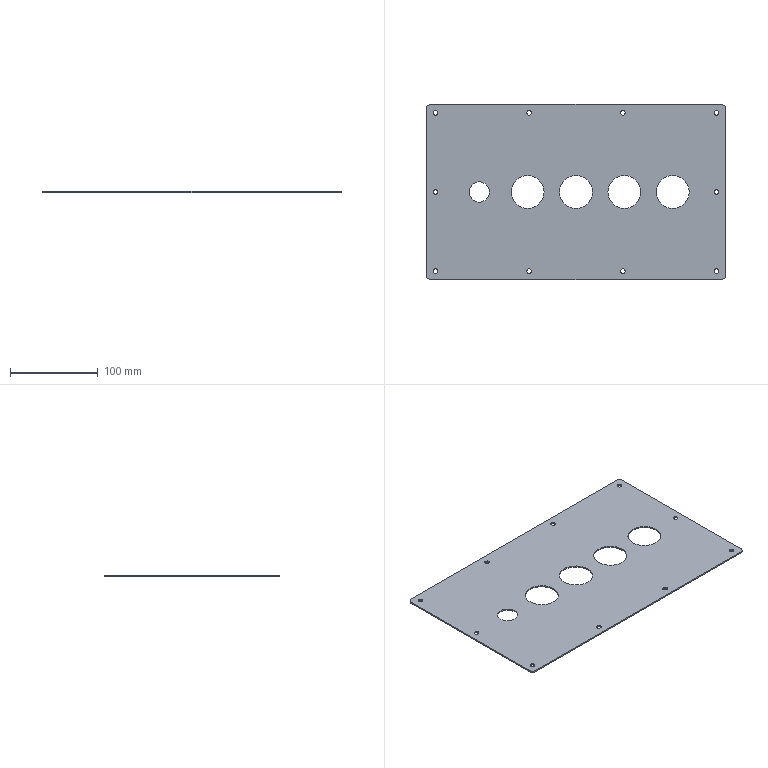Part | SolidWorks | features FlatPattern 1, SMBaseFlange 1, SheetMetal 1 | 1 solid | 40 faces | box 340 x 200 x 1.5 mm | volume 94399 mm3 | cylinder 34 | plane 6 | commonest cylinder face diameters 5.2 x20 37.5 x8 10 x4 23 x2
STEP:
#1=CARTESIAN_POINT('',(-12.59,100.,1.5));
#2=VERTEX_POINT('',#1);
#3=CARTESIAN_POINT('',(-7.39,100.,1.5));
#4=VERTEX_POINT('',#3);
#5=CARTESIAN_POINT('',(-9.99,100.,1.5));
#6=DIRECTION('',(0.,0.,1.));
#7=DIRECTION('',(1.,0.,0.));
#8=AXIS2_PLACEMENT_3D('',#5,#6,#7);
#9=CIRCLE('',#8,2.6);
#10=EDGE_CURVE('',#2,#4,#9,.T.);
#11=ORIENTED_EDGE('',*,*,#10,.T.);
#12=CARTESIAN_POINT('',(-7.39,100.,0.));
#13=VERTEX_POINT('',#12);
#14=CARTESIAN_POINT('',(-7.39,100.,1.5));
#15=DIRECTION('',(0.,0.,-1.));
#16=VECTOR('',#15,1000.);
#17=LINE('',#14,#16);
#18=EDGE_CURVE('',#4,#13,#17,.T.);
#19=ORIENTED_EDGE('',*,*,#18,.T.);
#20=CARTESIAN_POINT('',(-12.59,100.,0.));
#21=VERTEX_POINT('',#20);
#22=CARTESIAN_POINT('',(-9.99,100.,0.));
#23=DIRECTION('',(0.,0.,1.));
#24=DIRECTION('',(1.,0.,0.));
#25=AXIS2_PLACEMENT_3D('',#22,#23,#24);
#26=CIRCLE('',#25,2.6);
#27=EDGE_CURVE('',#21,#13,#26,.T.);
#28=ORIENTED_EDGE('',*,*,#27,.F.);
#29=CARTESIAN_POINT('',(-12.59,100.,1.5));
#30=DIRECTION('',(0.,0.,-1.));
#31=VECTOR('',#30,1000.);
#32=LINE('',#29,#31);
#33=EDGE_CURVE('',#2,#21,#32,.T.);
#34=ORIENTED_EDGE('',*,*,#33,.F.);
#35=EDGE_LOOP('',(#11,#19,#28,#34));
#36=FACE_OUTER_BOUND('',#35,.T.);
#37=CARTESIAN_POINT('',(-9.99,100.,1.5));
#38=DIRECTION('',(0.,0.,-1.));
#39=DIRECTION('',(-1.,0.,0.));
#40=AXIS2_PLACEMENT_3D('',#37,#38,#39);
#41=CYLINDRICAL_SURFACE('',#40,2.6);
#42=ADVANCED_FACE('',(#36),#41,.F.);
#43=CARTESIAN_POINT('',(-332.6,100.,1.5));
#44=VERTEX_POINT('',#43);
#45=CARTESIAN_POINT('',(-327.4,100.,1.5));
#46=VERTEX_POINT('',#45);
#47=CARTESIAN_POINT('',(-330.,100.,1.5));
#48=DIRECTION('',(0.,0.,1.));
#49=DIRECTION('',(1.,0.,0.));
#50=AXIS2_PLACEMENT_3D('',#47,#48,#49);
#51=CIRCLE('',#50,2.6);
#52=EDGE_CURVE('',#44,#46,#51,.T.);
#53=ORIENTED_EDGE('',*,*,#52,.T.);
#54=CARTESIAN_POINT('',(-327.4,100.,0.));
#55=VERTEX_POINT('',#54);
#56=CARTESIAN_POINT('',(-327.4,100.,1.5));
#57=DIRECTION('',(0.,0.,-1.));
#58=VECTOR('',#57,1000.);
#59=LINE('',#56,#58);
#60=EDGE_CURVE('',#46,#55,#59,.T.);
#61=ORIENTED_EDGE('',*,*,#60,.T.);
#62=CARTESIAN_POINT('',(-332.6,100.,0.));
#63=VERTEX_POINT('',#62);
#64=CARTESIAN_POINT('',(-330.,100.,0.));
#65=DIRECTION('',(0.,0.,1.));
#66=DIRECTION('',(1.,0.,0.));
#67=AXIS2_PLACEMENT_3D('',#64,#65,#66);
#68=CIRCLE('',#67,2.6);
#69=EDGE_CURVE('',#63,#55,#68,.T.);
#70=ORIENTED_EDGE('',*,*,#69,.F.);
#71=CARTESIAN_POINT('',(-332.6,100.,1.5));
#72=DIRECTION('',(0.,0.,-1.));
#73=VECTOR('',#72,1000.);
#74=LINE('',#71,#73);
#75=EDGE_CURVE('',#44,#63,#74,.T.);
#76=ORIENTED_EDGE('',*,*,#75,.F.);
#77=EDGE_LOOP('',(#53,#61,#70,#76));
#78=FACE_OUTER_BOUND('',#77,.T.);
#79=CARTESIAN_POINT('',(-330.,100.,1.5));
#80=DIRECTION('',(0.,0.,-1.));
#81=DIRECTION('',(-1.,0.,0.));
#82=AXIS2_PLACEMENT_3D('',#79,#80,#81);
#83=CYLINDRICAL_SURFACE('',#82,2.6);
#84=ADVANCED_FACE('',(#78),#83,.F.);
#85=CARTESIAN_POINT('',(-78.75,100.,1.5));
#86=VERTEX_POINT('',#85);
#87=CARTESIAN_POINT('',(-41.25,100.,1.5));
#88=VERTEX_POINT('',#87);
#89=CARTESIAN_POINT('',(-60.,100.,1.5));
#90=DIRECTION('',(0.,0.,1.));
#91=DIRECTION('',(1.,0.,0.));
#92=AXIS2_PLACEMENT_3D('',#89,#90,#91);
#93=CIRCLE('',#92,18.75);
#94=EDGE_CURVE('',#86,#88,#93,.T.);
#95=ORIENTED_EDGE('',*,*,#94,.T.);
#96=CARTESIAN_POINT('',(-41.25,100.,0.));
#97=VERTEX_POINT('',#96);
#98=CARTESIAN_POINT('',(-41.25,100.,1.5));
#99=DIRECTION('',(0.,0.,-1.));
#100=VECTOR('',#99,1000.);
#101=LINE('',#98,#100);
#102=EDGE_CURVE('',#88,#97,#101,.T.);
#103=ORIENTED_EDGE('',*,*,#102,.T.);
#104=CARTESIAN_POINT('',(-78.75,100.,0.));
#105=VERTEX_POINT('',#104);
#106=CARTESIAN_POINT('',(-60.,100.,0.));
#107=DIRECTION('',(0.,0.,1.));
#108=DIRECTION('',(1.,0.,0.));
#109=AXIS2_PLACEMENT_3D('',#106,#107,#108);
#110=CIRCLE('',#109,18.75);
#111=EDGE_CURVE('',#105,#97,#110,.T.);
#112=ORIENTED_EDGE('',*,*,#111,.F.);
#113=CARTESIAN_POINT('',(-78.75,100.,1.5));
#114=DIRECTION('',(0.,0.,-1.));
#115=VECTOR('',#114,1000.);
#116=LINE('',#113,#115);
#117=EDGE_CURVE('',#86,#105,#116,.T.);
#118=ORIENTED_EDGE('',*,*,#117,.F.);
#119=EDGE_LOOP('',(#95,#103,#112,#118));
#120=FACE_OUTER_BOUND('',#119,.T.);
#121=CARTESIAN_POINT('',(-60.,100.,1.5));
#122=DIRECTION('',(0.,0.,-1.));
#123=DIRECTION('',(-1.,0.,0.));
#124=AXIS2_PLACEMENT_3D('',#121,#122,#123);
#125=CYLINDRICAL_SURFACE('',#124,18.75);
#126=ADVANCED_FACE('',(#120),#125,.F.);
#127=CARTESIAN_POINT('',(-133.75,100.,1.5));
#128=VERTEX_POINT('',#127);
#129=CARTESIAN_POINT('',(-96.25,100.,1.5));
#130=VERTEX_POINT('',#129);
#131=CARTESIAN_POINT('',(-115.,100.,1.5));
#132=DIRECTION('',(0.,0.,1.));
#133=DIRECTION('',(1.,0.,0.));
#134=AXIS2_PLACEMENT_3D('',#131,#132,#133);
#135=CIRCLE('',#134,18.75);
#136=EDGE_CURVE('',#128,#130,#135,.T.);
#137=ORIENTED_EDGE('',*,*,#136,.T.);
#138=CARTESIAN_POINT('',(-96.25,100.,0.));
#139=VERTEX_POINT('',#138);
#140=CARTESIAN_POINT('',(-96.25,100.,1.5));
#141=DIRECTION('',(0.,0.,-1.));
#142=VECTOR('',#141,1000.);
#143=LINE('',#140,#142);
#144=EDGE_CURVE('',#130,#139,#143,.T.);
#145=ORIENTED_EDGE('',*,*,#144,.T.);
#146=CARTESIAN_POINT('',(-133.75,100.,0.));
#147=VERTEX_POINT('',#146);
#148=CARTESIAN_POINT('',(-115.,100.,0.));
#149=DIRECTION('',(0.,0.,1.));
#150=DIRECTION('',(1.,0.,0.));
#151=AXIS2_PLACEMENT_3D('',#148,#149,#150);
#152=CIRCLE('',#151,18.75);
#153=EDGE_CURVE('',#147,#139,#152,.T.);
#154=ORIENTED_EDGE('',*,*,#153,.F.);
#155=CARTESIAN_POINT('',(-133.75,100.,1.5));
#156=DIRECTION('',(0.,0.,-1.));
#157=VECTOR('',#156,1000.);
#158=LINE('',#155,#157);
#159=EDGE_CURVE('',#128,#147,#158,.T.);
#160=ORIENTED_EDGE('',*,*,#159,.F.);
#161=EDGE_LOOP('',(#137,#145,#154,#160));
#162=FACE_OUTER_BOUND('',#161,.T.);
#163=CARTESIAN_POINT('',(-115.,100.,1.5));
#164=DIRECTION('',(0.,0.,-1.));
#165=DIRECTION('',(-1.,0.,0.));
#166=AXIS2_PLACEMENT_3D('',#163,#164,#165);
#167=CYLINDRICAL_SURFACE('',#166,18.75);
#168=ADVANCED_FACE('',(#162),#167,.F.);
#169=CARTESIAN_POINT('',(-188.75,100.,1.5));
#170=VERTEX_POINT('',#169);
#171=CARTESIAN_POINT('',(-151.25,100.,1.5));
#172=VERTEX_POINT('',#171);
#173=CARTESIAN_POINT('',(-170.,100.,1.5));
#174=DIRECTION('',(0.,0.,1.));
#175=DIRECTION('',(1.,0.,0.));
#176=AXIS2_PLACEMENT_3D('',#173,#174,#175);
#177=CIRCLE('',#176,18.75);
#178=EDGE_CURVE('',#170,#172,#177,.T.);
#179=ORIENTED_EDGE('',*,*,#178,.T.);
#180=CARTESIAN_POINT('',(-151.25,100.,0.));
#181=VERTEX_POINT('',#180);
#182=CARTESIAN_POINT('',(-151.25,100.,1.5));
#183=DIRECTION('',(0.,0.,-1.));
#184=VECTOR('',#183,1000.);
#185=LINE('',#182,#184);
#186=EDGE_CURVE('',#172,#181,#185,.T.);
#187=ORIENTED_EDGE('',*,*,#186,.T.);
#188=CARTESIAN_POINT('',(-188.75,100.,0.));
#189=VERTEX_POINT('',#188);
#190=CARTESIAN_POINT('',(-170.,100.,0.));
#191=DIRECTION('',(0.,0.,1.));
#192=DIRECTION('',(1.,0.,0.));
#193=AXIS2_PLACEMENT_3D('',#190,#191,#192);
#194=CIRCLE('',#193,18.75);
#195=EDGE_CURVE('',#189,#181,#194,.T.);
#196=ORIENTED_EDGE('',*,*,#195,.F.);
#197=CARTESIAN_POINT('',(-188.75,100.,1.5));
#198=DIRECTION('',(0.,0.,-1.));
#199=VECTOR('',#198,1000.);
#200=LINE('',#197,#199);
#201=EDGE_CURVE('',#170,#189,#200,.T.);
#202=ORIENTED_EDGE('',*,*,#201,.F.);
#203=EDGE_LOOP('',(#179,#187,#196,#202));
#204=FACE_OUTER_BOUND('',#203,.T.);
#205=CARTESIAN_POINT('',(-170.,100.,1.5));
#206=DIRECTION('',(0.,0.,-1.));
#207=DIRECTION('',(-1.,0.,0.));
#208=AXIS2_PLACEMENT_3D('',#205,#206,#207);
#209=CYLINDRICAL_SURFACE('',#208,18.75);
#210=ADVANCED_FACE('',(#204),#209,.F.);
#211=CARTESIAN_POINT('',(-243.75,100.,1.5));
#212=VERTEX_POINT('',#211);
#213=CARTESIAN_POINT('',(-206.25,100.,1.5));
#214=VERTEX_POINT('',#213);
#215=CARTESIAN_POINT('',(-225.,100.,1.5));
#216=DIRECTION('',(0.,0.,1.));
#217=DIRECTION('',(1.,0.,0.));
#218=AXIS2_PLACEMENT_3D('',#215,#216,#217);
#219=CIRCLE('',#218,18.75);
#220=EDGE_CURVE('',#212,#214,#219,.T.);
#221=ORIENTED_EDGE('',*,*,#220,.T.);
#222=CARTESIAN_POINT('',(-206.25,100.,0.));
#223=VERTEX_POINT('',#222);
#224=CARTESIAN_POINT('',(-206.25,100.,1.5));
#225=DIRECTION('',(0.,0.,-1.));
#226=VECTOR('',#225,1000.);
#227=LINE('',#224,#226);
#228=EDGE_CURVE('',#214,#223,#227,.T.);
#229=ORIENTED_EDGE('',*,*,#228,.T.);
#230=CARTESIAN_POINT('',(-243.75,100.,0.));
#231=VERTEX_POINT('',#230);
#232=CARTESIAN_POINT('',(-225.,100.,0.));
#233=DIRECTION('',(0.,0.,1.));
#234=DIRECTION('',(1.,0.,0.));
#235=AXIS2_PLACEMENT_3D('',#232,#233,#234);
#236=CIRCLE('',#235,18.75);
#237=EDGE_CURVE('',#231,#223,#236,.T.);
#238=ORIENTED_EDGE('',*,*,#237,.F.);
#239=CARTESIAN_POINT('',(-243.75,100.,1.5));
#240=DIRECTION('',(0.,0.,-1.));
#241=VECTOR('',#240,1000.);
#242=LINE('',#239,#241);
#243=EDGE_CURVE('',#212,#231,#242,.T.);
#244=ORIENTED_EDGE('',*,*,#243,.F.);
#245=EDGE_LOOP('',(#221,#229,#238,#244));
#246=FACE_OUTER_BOUND('',#245,.T.);
#247=CARTESIAN_POINT('',(-225.,100.,1.5));
#248=DIRECTION('',(0.,0.,-1.));
#249=DIRECTION('',(-1.,0.,0.));
#250=AXIS2_PLACEMENT_3D('',#247,#248,#249);
#251=CYLINDRICAL_SURFACE('',#250,18.75);
#252=ADVANCED_FACE('',(#246),#251,.F.);
#253=CARTESIAN_POINT('',(-291.5,100.,1.5));
#254=VERTEX_POINT('',#253);
#255=CARTESIAN_POINT('',(-268.5,100.,1.5));
#256=VERTEX_POINT('',#255);
#257=CARTESIAN_POINT('',(-280.,100.,1.5));
#258=DIRECTION('',(0.,0.,1.));
#259=DIRECTION('',(1.,0.,0.));
#260=AXIS2_PLACEMENT_3D('',#257,#258,#259);
#261=CIRCLE('',#260,11.5);
#262=EDGE_CURVE('',#254,#256,#261,.T.);
#263=ORIENTED_EDGE('',*,*,#262,.T.);
#264=CARTESIAN_POINT('',(-268.5,100.,0.));
#265=VERTEX_POINT('',#264);
#266=CARTESIAN_POINT('',(-268.5,100.,1.5));
#267=DIRECTION('',(0.,0.,-1.));
#268=VECTOR('',#267,1000.);
#269=LINE('',#266,#268);
#270=EDGE_CURVE('',#256,#265,#269,.T.);
#271=ORIENTED_EDGE('',*,*,#270,.T.);
#272=CARTESIAN_POINT('',(-291.5,100.,0.));
#273=VERTEX_POINT('',#272);
#274=CARTESIAN_POINT('',(-280.,100.,0.));
#275=DIRECTION('',(0.,0.,1.));
#276=DIRECTION('',(1.,0.,0.));
#277=AXIS2_PLACEMENT_3D('',#274,#275,#276);
#278=CIRCLE('',#277,11.5);
#279=EDGE_CURVE('',#273,#265,#278,.T.);
#280=ORIENTED_EDGE('',*,*,#279,.F.);
#281=CARTESIAN_POINT('',(-291.5,100.,1.5));
#282=DIRECTION('',(0.,0.,-1.));
#283=VECTOR('',#282,1000.);
#284=LINE('',#281,#283);
#285=EDGE_CURVE('',#254,#273,#284,.T.);
#286=ORIENTED_EDGE('',*,*,#285,.F.);
#287=EDGE_LOOP('',(#263,#271,#280,#286));
#288=FACE_OUTER_BOUND('',#287,.T.);
#289=CARTESIAN_POINT('',(-280.,100.,1.5));
#290=DIRECTION('',(0.,0.,-1.));
#291=DIRECTION('',(-1.,0.,0.));
#292=AXIS2_PLACEMENT_3D('',#289,#290,#291);
#293=CYLINDRICAL_SURFACE('',#292,11.5);
#294=ADVANCED_FACE('',(#288),#293,.F.);
#295=CARTESIAN_POINT('',(-12.59,10.,1.5));
#296=VERTEX_POINT('',#295);
#297=CARTESIAN_POINT('',(-7.39,10.,1.5));
#298=VERTEX_POINT('',#297);
#299=CARTESIAN_POINT('',(-9.99,10.,1.5));
#300=DIRECTION('',(0.,0.,1.));
#301=DIRECTION('',(1.,0.,0.));
#302=AXIS2_PLACEMENT_3D('',#299,#300,#301);
#303=CIRCLE('',#302,2.6);
#304=EDGE_CURVE('',#296,#298,#303,.T.);
#305=ORIENTED_EDGE('',*,*,#304,.T.);
#306=CARTESIAN_POINT('',(-7.39,10.,0.));
#307=VERTEX_POINT('',#306);
#308=CARTESIAN_POINT('',(-7.39,10.,1.5));
#309=DIRECTION('',(0.,0.,-1.));
#310=VECTOR('',#309,1000.);
#311=LINE('',#308,#310);
#312=EDGE_CURVE('',#298,#307,#311,.T.);
#313=ORIENTED_EDGE('',*,*,#312,.T.);
#314=CARTESIAN_POINT('',(-12.59,10.,0.));
#315=VERTEX_POINT('',#314);
#316=CARTESIAN_POINT('',(-9.99,10.,0.));
#317=DIRECTION('',(0.,0.,1.));
#318=DIRECTION('',(1.,0.,0.));
#319=AXIS2_PLACEMENT_3D('',#316,#317,#318);
#320=CIRCLE('',#319,2.6);
#321=EDGE_CURVE('',#315,#307,#320,.T.);
#322=ORIENTED_EDGE('',*,*,#321,.F.);
#323=CARTESIAN_POINT('',(-12.59,10.,1.5));
#324=DIRECTION('',(0.,0.,-1.));
#325=VECTOR('',#324,1000.);
#326=LINE('',#323,#325);
#327=EDGE_CURVE('',#296,#315,#326,.T.);
#328=ORIENTED_EDGE('',*,*,#327,.F.);
#329=EDGE_LOOP('',(#305,#313,#322,#328));
#330=FACE_OUTER_BOUND('',#329,.T.);
#331=CARTESIAN_POINT('',(-9.99,10.,1.5));
#332=DIRECTION('',(0.,0.,-1.));
#333=DIRECTION('',(-1.,0.,0.));
#334=AXIS2_PLACEMENT_3D('',#331,#332,#333);
#335=CYLINDRICAL_SURFACE('',#334,2.6);
#336=ADVANCED_FACE('',(#330),#335,.F.);
#337=CARTESIAN_POINT('',(-119.26,10.,1.5));
#338=VERTEX_POINT('',#337);
#339=CARTESIAN_POINT('',(-114.06,10.,1.5));
#340=VERTEX_POINT('',#339);
#341=CARTESIAN_POINT('',(-116.66,10.,1.5));
#342=DIRECTION('',(0.,0.,1.));
#343=DIRECTION('',(1.,0.,0.));
#344=AXIS2_PLACEMENT_3D('',#341,#342,#343);
#345=CIRCLE('',#344,2.6);
#346=EDGE_CURVE('',#338,#340,#345,.T.);
#347=ORIENTED_EDGE('',*,*,#346,.T.);
#348=CARTESIAN_POINT('',(-114.06,10.,0.));
#349=VERTEX_POINT('',#348);
#350=CARTESIAN_POINT('',(-114.06,10.,1.5));
#351=DIRECTION('',(0.,0.,-1.));
#352=VECTOR('',#351,1000.);
#353=LINE('',#350,#352);
#354=EDGE_CURVE('',#340,#349,#353,.T.);
#355=ORIENTED_EDGE('',*,*,#354,.T.);
#356=CARTESIAN_POINT('',(-119.26,10.,0.));
#357=VERTEX_POINT('',#356);
#358=CARTESIAN_POINT('',(-116.66,10.,0.));
#359=DIRECTION('',(0.,0.,1.));
#360=DIRECTION('',(1.,0.,0.));
#361=AXIS2_PLACEMENT_3D('',#358,#359,#360);
#362=CIRCLE('',#361,2.6);
#363=EDGE_CURVE('',#357,#349,#362,.T.);
#364=ORIENTED_EDGE('',*,*,#363,.F.);
#365=CARTESIAN_POINT('',(-119.26,10.,1.5));
#366=DIRECTION('',(0.,0.,-1.));
#367=VECTOR('',#366,1000.);
#368=LINE('',#365,#367);
#369=EDGE_CURVE('',#338,#357,#368,.T.);
#370=ORIENTED_EDGE('',*,*,#369,.F.);
#371=EDGE_LOOP('',(#347,#355,#364,#370));
#372=FACE_OUTER_BOUND('',#371,.T.);
#373=CARTESIAN_POINT('',(-116.66,10.,1.5));
#374=DIRECTION('',(0.,0.,-1.));
#375=DIRECTION('',(-1.,0.,0.));
#376=AXIS2_PLACEMENT_3D('',#373,#374,#375);
#377=CYLINDRICAL_SURFACE('',#376,2.6);
#378=ADVANCED_FACE('',(#372),#377,.F.);
#379=CARTESIAN_POINT('',(-225.93,10.,1.5));
#380=VERTEX_POINT('',#379);
#381=CARTESIAN_POINT('',(-220.73,10.,1.5));
#382=VERTEX_POINT('',#381);
#383=CARTESIAN_POINT('',(-223.33,10.,1.5));
#384=DIRECTION('',(0.,0.,1.));
#385=DIRECTION('',(1.,0.,0.));
#386=AXIS2_PLACEMENT_3D('',#383,#384,#385);
#387=CIRCLE('',#386,2.6);
#388=EDGE_CURVE('',#380,#382,#387,.T.);
#389=ORIENTED_EDGE('',*,*,#388,.T.);
#390=CARTESIAN_POINT('',(-220.73,10.,0.));
#391=VERTEX_POINT('',#390);
#392=CARTESIAN_POINT('',(-220.73,10.,1.5));
#393=DIRECTION('',(0.,0.,-1.));
#394=VECTOR('',#393,1000.);
#395=LINE('',#392,#394);
#396=EDGE_CURVE('',#382,#391,#395,.T.);
#397=ORIENTED_EDGE('',*,*,#396,.T.);
#398=CARTESIAN_POINT('',(-225.93,10.,0.));
#399=VERTEX_POINT('',#398);
#400=CARTESIAN_POINT('',(-223.33,10.,0.));
#401=DIRECTION('',(0.,0.,1.));
#402=DIRECTION('',(1.,0.,0.));
#403=AXIS2_PLACEMENT_3D('',#400,#401,#402);
#404=CIRCLE('',#403,2.6);
#405=EDGE_CURVE('',#399,#391,#404,.T.);
#406=ORIENTED_EDGE('',*,*,#405,.F.);
#407=CARTESIAN_POINT('',(-225.93,10.,1.5));
#408=DIRECTION('',(0.,0.,-1.));
#409=VECTOR('',#408,1000.);
#410=LINE('',#407,#409);
#411=EDGE_CURVE('',#380,#399,#410,.T.);
#412=ORIENTED_EDGE('',*,*,#411,.F.);
#413=EDGE_LOOP('',(#389,#397,#406,#412));
#414=FACE_OUTER_BOUND('',#413,.T.);
#415=CARTESIAN_POINT('',(-223.33,10.,1.5));
#416=DIRECTION('',(0.,0.,-1.));
#417=DIRECTION('',(-1.,0.,0.));
#418=AXIS2_PLACEMENT_3D('',#415,#416,#417);
#419=CYLINDRICAL_SURFACE('',#418,2.6);
#420=ADVANCED_FACE('',(#414),#419,.F.);
#421=CARTESIAN_POINT('',(-332.6,10.,1.5));
#422=VERTEX_POINT('',#421);
#423=CARTESIAN_POINT('',(-327.4,10.,1.5));
#424=VERTEX_POINT('',#423);
#425=CARTESIAN_POINT('',(-330.,10.,1.5));
#426=DIRECTION('',(0.,0.,1.));
#427=DIRECTION('',(1.,0.,0.));
#428=AXIS2_PLACEMENT_3D('',#425,#426,#427);
#429=CIRCLE('',#428,2.6);
#430=EDGE_CURVE('',#422,#424,#429,.T.);
#431=ORIENTED_EDGE('',*,*,#430,.T.);
#432=CARTESIAN_POINT('',(-327.4,10.,0.));
#433=VERTEX_POINT('',#432);
#434=CARTESIAN_POINT('',(-327.4,10.,1.5));
#435=DIRECTION('',(0.,0.,-1.));
#436=VECTOR('',#435,1000.);
#437=LINE('',#434,#436);
#438=EDGE_CURVE('',#424,#433,#437,.T.);
#439=ORIENTED_EDGE('',*,*,#438,.T.);
#440=CARTESIAN_POINT('',(-332.6,10.,0.));
#441=VERTEX_POINT('',#440);
#442=CARTESIAN_POINT('',(-330.,10.,0.));
#443=DIRECTION('',(0.,0.,1.));
#444=DIRECTION('',(1.,0.,0.));
#445=AXIS2_PLACEMENT_3D('',#442,#443,#444);
#446=CIRCLE('',#445,2.6);
#447=EDGE_CURVE('',#441,#433,#446,.T.);
#448=ORIENTED_EDGE('',*,*,#447,.F.);
#449=CARTESIAN_POINT('',(-332.6,10.,1.5));
#450=DIRECTION('',(0.,0.,-1.));
#451=VECTOR('',#450,1000.);
#452=LINE('',#449,#451);
#453=EDGE_CURVE('',#422,#441,#452,.T.);
#454=ORIENTED_EDGE('',*,*,#453,.F.);
#455=EDGE_LOOP('',(#431,#439,#448,#454));
#456=FACE_OUTER_BOUND('',#455,.T.);
#457=CARTESIAN_POINT('',(-330.,10.,1.5));
#458=DIRECTION('',(0.,0.,-1.));
#459=DIRECTION('',(-1.,0.,0.));
#460=AXIS2_PLACEMENT_3D('',#457,#458,#459);
#461=CYLINDRICAL_SURFACE('',#460,2.6);
#462=ADVANCED_FACE('',(#456),#461,.F.);
#463=CARTESIAN_POINT('',(-12.59,190.,1.5));
#464=VERTEX_POINT('',#463);
#465=CARTESIAN_POINT('',(-7.39,190.,1.5));
#466=VERTEX_POINT('',#465);
#467=CARTESIAN_POINT('',(-9.99,190.,1.5));
#468=DIRECTION('',(0.,0.,1.));
#469=DIRECTION('',(1.,0.,0.));
#470=AXIS2_PLACEMENT_3D('',#467,#468,#469);
#471=CIRCLE('',#470,2.6);
#472=EDGE_CURVE('',#464,#466,#471,.T.);
#473=ORIENTED_EDGE('',*,*,#472,.T.);
#474=CARTESIAN_POINT('',(-7.39,190.,0.));
#475=VERTEX_POINT('',#474);
#476=CARTESIAN_POINT('',(-7.39,190.,1.5));
#477=DIRECTION('',(0.,0.,-1.));
#478=VECTOR('',#477,1000.);
#479=LINE('',#476,#478);
#480=EDGE_CURVE('',#466,#475,#479,.T.);
#481=ORIENTED_EDGE('',*,*,#480,.T.);
#482=CARTESIAN_POINT('',(-12.59,190.,0.));
#483=VERTEX_POINT('',#482);
#484=CARTESIAN_POINT('',(-9.99,190.,0.));
#485=DIRECTION('',(0.,0.,1.));
#486=DIRECTION('',(1.,0.,0.));
#487=AXIS2_PLACEMENT_3D('',#484,#485,#486);
#488=CIRCLE('',#487,2.6);
#489=EDGE_CURVE('',#483,#475,#488,.T.);
#490=ORIENTED_EDGE('',*,*,#489,.F.);
#491=CARTESIAN_POINT('',(-12.59,190.,1.5));
#492=DIRECTION('',(0.,0.,-1.));
#493=VECTOR('',#492,1000.);
#494=LINE('',#491,#493);
#495=EDGE_CURVE('',#464,#483,#494,.T.);
#496=ORIENTED_EDGE('',*,*,#495,.F.);
#497=EDGE_LOOP('',(#473,#481,#490,#496));
#498=FACE_OUTER_BOUND('',#497,.T.);
#499=CARTESIAN_POINT('',(-9.99,190.,1.5));
#500=DIRECTION('',(0.,0.,-1.));
#501=DIRECTION('',(-1.,0.,0.));
#502=AXIS2_PLACEMENT_3D('',#499,#500,#501);
#503=CYLINDRICAL_SURFACE('',#502,2.6);
#504=ADVANCED_FACE('',(#498),#503,.F.);
#505=CARTESIAN_POINT('',(-119.26,190.,1.5));
#506=VERTEX_POINT('',#505);
#507=CARTESIAN_POINT('',(-114.06,190.,1.5));
#508=VERTEX_POINT('',#507);
#509=CARTESIAN_POINT('',(-116.66,190.,1.5));
#510=DIRECTION('',(0.,0.,1.));
#511=DIRECTION('',(1.,0.,0.));
#512=AXIS2_PLACEMENT_3D('',#509,#510,#511);
#513=CIRCLE('',#512,2.6);
#514=EDGE_CURVE('',#506,#508,#513,.T.);
#515=ORIENTED_EDGE('',*,*,#514,.T.);
#516=CARTESIAN_POINT('',(-114.06,190.,0.));
#517=VERTEX_POINT('',#516);
#518=CARTESIAN_POINT('',(-114.06,190.,1.5));
#519=DIRECTION('',(0.,0.,-1.));
#520=VECTOR('',#519,1000.);
#521=LINE('',#518,#520);
#522=EDGE_CURVE('',#508,#517,#521,.T.);
#523=ORIENTED_EDGE('',*,*,#522,.T.);
#524=CARTESIAN_POINT('',(-119.26,190.,0.));
#525=VERTEX_POINT('',#524);
#526=CARTESIAN_POINT('',(-116.66,190.,0.));
#527=DIRECTION('',(0.,0.,1.));
#528=DIRECTION('',(1.,0.,0.));
#529=AXIS2_PLACEMENT_3D('',#526,#527,#528);
#530=CIRCLE('',#529,2.6);
#531=EDGE_CURVE('',#525,#517,#530,.T.);
#532=ORIENTED_EDGE('',*,*,#531,.F.);
#533=CARTESIAN_POINT('',(-119.26,190.,1.5));
#534=DIRECTION('',(0.,0.,-1.));
#535=VECTOR('',#534,1000.);
#536=LINE('',#533,#535);
#537=EDGE_CURVE('',#506,#525,#536,.T.);
#538=ORIENTED_EDGE('',*,*,#537,.F.);
#539=EDGE_LOOP('',(#515,#523,#532,#538));
#540=FACE_OUTER_BOUND('',#539,.T.);
#541=CARTESIAN_POINT('',(-116.66,190.,1.5));
#542=DIRECTION('',(0.,0.,-1.));
#543=DIRECTION('',(-1.,0.,0.));
#544=AXIS2_PLACEMENT_3D('',#541,#542,#543);
#545=CYLINDRICAL_SURFACE('',#544,2.6);
#546=ADVANCED_FACE('',(#540),#545,.F.);
#547=CARTESIAN_POINT('',(-225.93,190.,1.5));
#548=VERTEX_POINT('',#547);
#549=CARTESIAN_POINT('',(-220.73,190.,1.5));
#550=VERTEX_POINT('',#549);
#551=CARTESIAN_POINT('',(-223.33,190.,1.5));
#552=DIRECTION('',(0.,0.,1.));
#553=DIRECTION('',(1.,0.,0.));
#554=AXIS2_PLACEMENT_3D('',#551,#552,#553);
#555=CIRCLE('',#554,2.6);
#556=EDGE_CURVE('',#548,#550,#555,.T.);
#557=ORIENTED_EDGE('',*,*,#556,.T.);
#558=CARTESIAN_POINT('',(-220.73,190.,0.));
#559=VERTEX_POINT('',#558);
#560=CARTESIAN_POINT('',(-220.73,190.,1.5));
#561=DIRECTION('',(0.,0.,-1.));
#562=VECTOR('',#561,1000.);
#563=LINE('',#560,#562);
#564=EDGE_CURVE('',#550,#559,#563,.T.);
#565=ORIENTED_EDGE('',*,*,#564,.T.);
#566=CARTESIAN_POINT('',(-225.93,190.,0.));
#567=VERTEX_POINT('',#566);
#568=CARTESIAN_POINT('',(-223.33,190.,0.));
#569=DIRECTION('',(0.,0.,1.));
#570=DIRECTION('',(1.,0.,0.));
#571=AXIS2_PLACEMENT_3D('',#568,#569,#570);
#572=CIRCLE('',#571,2.6);
#573=EDGE_CURVE('',#567,#559,#572,.T.);
#574=ORIENTED_EDGE('',*,*,#573,.F.);
#575=CARTESIAN_POINT('',(-225.93,190.,1.5));
#576=DIRECTION('',(0.,0.,-1.));
#577=VECTOR('',#576,1000.);
#578=LINE('',#575,#577);
#579=EDGE_CURVE('',#548,#567,#578,.T.);
#580=ORIENTED_EDGE('',*,*,#579,.F.);
#581=EDGE_LOOP('',(#557,#565,#574,#580));
#582=FACE_OUTER_BOUND('',#581,.T.);
#583=CARTESIAN_POINT('',(-223.33,190.,1.5));
#584=DIRECTION('',(0.,0.,-1.));
#585=DIRECTION('',(-1.,0.,0.));
#586=AXIS2_PLACEMENT_3D('',#583,#584,#585);
#587=CYLINDRICAL_SURFACE('',#586,2.6);
#588=ADVANCED_FACE('',(#582),#587,.F.);
#589=CARTESIAN_POINT('',(-332.6,190.,1.5));
#590=VERTEX_POINT('',#589);
#591=CARTESIAN_POINT('',(-327.4,190.,1.5));
#592=VERTEX_POINT('',#591);
#593=CARTESIAN_POINT('',(-330.,190.,1.5));
#594=DIRECTION('',(0.,0.,1.));
#595=DIRECTION('',(1.,0.,0.));
#596=AXIS2_PLACEMENT_3D('',#593,#594,#595);
#597=CIRCLE('',#596,2.6);
#598=EDGE_CURVE('',#590,#592,#597,.T.);
#599=ORIENTED_EDGE('',*,*,#598,.T.);
#600=CARTESIAN_POINT('',(-327.4,190.,0.));
#601=VERTEX_POINT('',#600);
#602=CARTESIAN_POINT('',(-327.4,190.,1.5));
#603=DIRECTION('',(0.,0.,-1.));
#604=VECTOR('',#603,1000.);
#605=LINE('',#602,#604);
#606=EDGE_CURVE('',#592,#601,#605,.T.);
#607=ORIENTED_EDGE('',*,*,#606,.T.);
#608=CARTESIAN_POINT('',(-332.6,190.,0.));
#609=VERTEX_POINT('',#608);
#610=CARTESIAN_POINT('',(-330.,190.,0.));
#611=DIRECTION('',(0.,0.,1.));
#612=DIRECTION('',(1.,0.,0.));
#613=AXIS2_PLACEMENT_3D('',#610,#611,#612);
#614=CIRCLE('',#613,2.6);
#615=EDGE_CURVE('',#609,#601,#614,.T.);
#616=ORIENTED_EDGE('',*,*,#615,.F.);
#617=CARTESIAN_POINT('',(-332.6,190.,1.5));
#618=DIRECTION('',(0.,0.,-1.));
#619=VECTOR('',#618,1000.);
#620=LINE('',#617,#619);
#621=EDGE_CURVE('',#590,#609,#620,.T.);
#622=ORIENTED_EDGE('',*,*,#621,.F.);
#623=EDGE_LOOP('',(#599,#607,#616,#622));
#624=FACE_OUTER_BOUND('',#623,.T.);
#625=CARTESIAN_POINT('',(-330.,190.,1.5));
#626=DIRECTION('',(0.,0.,-1.));
#627=DIRECTION('',(-1.,0.,0.));
#628=AXIS2_PLACEMENT_3D('',#625,#626,#627);
#629=CYLINDRICAL_SURFACE('',#628,2.6);
#630=ADVANCED_FACE('',(#624),#629,.F.);
#631=ORIENTED_EDGE('',*,*,#52,.F.);
#632=CARTESIAN_POINT('',(-330.,100.,1.5));
#633=DIRECTION('',(0.,0.,1.));
#634=DIRECTION('',(1.,0.,0.));
#635=AXIS2_PLACEMENT_3D('',#632,#633,#634);
#636=CIRCLE('',#635,2.6);
#637=EDGE_CURVE('',#46,#44,#636,.T.);
#638=ORIENTED_EDGE('',*,*,#637,.F.);
#639=EDGE_LOOP('',(#631,#638));
#640=FACE_BOUND('',#639,.T.);
#641=ORIENTED_EDGE('',*,*,#136,.F.);
#642=CARTESIAN_POINT('',(-115.,100.,1.5));
#643=DIRECTION('',(0.,0.,1.));
#644=DIRECTION('',(1.,0.,0.));
#645=AXIS2_PLACEMENT_3D('',#642,#643,#644);
#646=CIRCLE('',#645,18.75);
#647=EDGE_CURVE('',#130,#128,#646,.T.);
#648=ORIENTED_EDGE('',*,*,#647,.F.);
#649=EDGE_LOOP('',(#641,#648));
#650=FACE_BOUND('',#649,.T.);
#651=ORIENTED_EDGE('',*,*,#220,.F.);
#652=CARTESIAN_POINT('',(-225.,100.,1.5));
#653=DIRECTION('',(0.,0.,1.));
#654=DIRECTION('',(1.,0.,0.));
#655=AXIS2_PLACEMENT_3D('',#652,#653,#654);
#656=CIRCLE('',#655,18.75);
#657=EDGE_CURVE('',#214,#212,#656,.T.);
#658=ORIENTED_EDGE('',*,*,#657,.F.);
#659=EDGE_LOOP('',(#651,#658));
#660=FACE_BOUND('',#659,.T.);
#661=ORIENTED_EDGE('',*,*,#304,.F.);
#662=CARTESIAN_POINT('',(-9.99,10.,1.5));
#663=DIRECTION('',(0.,0.,1.));
#664=DIRECTION('',(1.,0.,0.));
#665=AXIS2_PLACEMENT_3D('',#662,#663,#664);
#666=CIRCLE('',#665,2.6);
#667=EDGE_CURVE('',#298,#296,#666,.T.);
#668=ORIENTED_EDGE('',*,*,#667,.F.);
#669=EDGE_LOOP('',(#661,#668));
#670=FACE_BOUND('',#669,.T.);
#671=ORIENTED_EDGE('',*,*,#388,.F.);
#672=CARTESIAN_POINT('',(-223.33,10.,1.5));
#673=DIRECTION('',(0.,0.,1.));
#674=DIRECTION('',(1.,0.,0.));
#675=AXIS2_PLACEMENT_3D('',#672,#673,#674);
#676=CIRCLE('',#675,2.6);
#677=EDGE_CURVE('',#382,#380,#676,.T.);
#678=ORIENTED_EDGE('',*,*,#677,.F.);
#679=EDGE_LOOP('',(#671,#678));
#680=FACE_BOUND('',#679,.T.);
#681=ORIENTED_EDGE('',*,*,#472,.F.);
#682=CARTESIAN_POINT('',(-9.99,190.,1.5));
#683=DIRECTION('',(0.,0.,1.));
#684=DIRECTION('',(1.,0.,0.));
#685=AXIS2_PLACEMENT_3D('',#682,#683,#684);
#686=CIRCLE('',#685,2.6);
#687=EDGE_CURVE('',#466,#464,#686,.T.);
#688=ORIENTED_EDGE('',*,*,#687,.F.);
#689=EDGE_LOOP('',(#681,#688));
#690=FACE_BOUND('',#689,.T.);
#691=ORIENTED_EDGE('',*,*,#556,.F.);
#692=CARTESIAN_POINT('',(-223.33,190.,1.5));
#693=DIRECTION('',(0.,0.,1.));
#694=DIRECTION('',(1.,0.,0.));
#695=AXIS2_PLACEMENT_3D('',#692,#693,#694);
#696=CIRCLE('',#695,2.6);
#697=EDGE_CURVE('',#550,#548,#696,.T.);
#698=ORIENTED_EDGE('',*,*,#697,.F.);
#699=EDGE_LOOP('',(#691,#698));
#700=FACE_BOUND('',#699,.T.);
#701=CARTESIAN_POINT('',(-335.,200.,1.5));
#702=VERTEX_POINT('',#701);
#703=CARTESIAN_POINT('',(-340.,195.,1.5));
#704=VERTEX_POINT('',#703);
#705=CARTESIAN_POINT('',(-335.,195.,1.5));
#706=DIRECTION('',(0.,0.,1.));
#707=DIRECTION('',(1.,0.,0.));
#708=AXIS2_PLACEMENT_3D('',#705,#706,#707);
#709=CIRCLE('',#708,5.);
#710=EDGE_CURVE('',#702,#704,#709,.T.);
#711=ORIENTED_EDGE('',*,*,#710,.T.);
#712=CARTESIAN_POINT('',(-340.,5.,1.5));
#713=VERTEX_POINT('',#712);
#714=CARTESIAN_POINT('',(-340.,5.,1.5));
#715=DIRECTION('',(0.,-1.,0.));
#716=VECTOR('',#715,1000.);
#717=LINE('',#714,#716);
#718=EDGE_CURVE('',#704,#713,#717,.T.);
#719=ORIENTED_EDGE('',*,*,#718,.T.);
#720=CARTESIAN_POINT('',(-335.,0.,1.5));
#721=VERTEX_POINT('',#720);
#722=CARTESIAN_POINT('',(-335.,5.,1.5));
#723=DIRECTION('',(0.,0.,1.));
#724=DIRECTION('',(-1.,0.,0.));
#725=AXIS2_PLACEMENT_3D('',#722,#723,#724);
#726=CIRCLE('',#725,5.);
#727=EDGE_CURVE('',#713,#721,#726,.T.);
#728=ORIENTED_EDGE('',*,*,#727,.T.);
#729=CARTESIAN_POINT('',(-5.,0.,1.5));
#730=VERTEX_POINT('',#729);
#731=CARTESIAN_POINT('',(-5.,0.,1.5));
#732=DIRECTION('',(1.,0.,0.));
#733=VECTOR('',#732,1000.);
#734=LINE('',#731,#733);
#735=EDGE_CURVE('',#721,#730,#734,.T.);
#736=ORIENTED_EDGE('',*,*,#735,.T.);
#737=CARTESIAN_POINT('',(0.,5.,1.5));
#738=VERTEX_POINT('',#737);
#739=CARTESIAN_POINT('',(-5.,5.,1.5));
#740=DIRECTION('',(0.,0.,1.));
#741=DIRECTION('',(1.,0.,0.));
#742=AXIS2_PLACEMENT_3D('',#739,#740,#741);
#743=CIRCLE('',#742,5.);
#744=EDGE_CURVE('',#730,#738,#743,.T.);
#745=ORIENTED_EDGE('',*,*,#744,.T.);
#746=CARTESIAN_POINT('',(0.,195.,1.5));
#747=VERTEX_POINT('',#746);
#748=CARTESIAN_POINT('',(0.,5.,1.5));
#749=DIRECTION('',(0.,1.,0.));
#750=VECTOR('',#749,1000.);
#751=LINE('',#748,#750);
#752=EDGE_CURVE('',#738,#747,#751,.T.);
#753=ORIENTED_EDGE('',*,*,#752,.T.);
#754=CARTESIAN_POINT('',(-5.,200.,1.5));
#755=VERTEX_POINT('',#754);
#756=CARTESIAN_POINT('',(-5.,195.,1.5));
#757=DIRECTION('',(0.,0.,1.));
#758=DIRECTION('',(1.,0.,0.));
#759=AXIS2_PLACEMENT_3D('',#756,#757,#758);
#760=CIRCLE('',#759,5.);
#761=EDGE_CURVE('',#747,#755,#760,.T.);
#762=ORIENTED_EDGE('',*,*,#761,.T.);
#763=CARTESIAN_POINT('',(-5.,200.,1.5));
#764=DIRECTION('',(-1.,0.,0.));
#765=VECTOR('',#764,1000.);
#766=LINE('',#763,#765);
#767=EDGE_CURVE('',#755,#702,#766,.T.);
#768=ORIENTED_EDGE('',*,*,#767,.T.);
#769=EDGE_LOOP('',(#711,#719,#728,#736,#745,#753,#762,#768));
#770=FACE_OUTER_BOUND('',#769,.T.);
#771=ORIENTED_EDGE('',*,*,#598,.F.);
#772=CARTESIAN_POINT('',(-330.,190.,1.5));
#773=DIRECTION('',(0.,0.,1.));
#774=DIRECTION('',(1.,0.,0.));
#775=AXIS2_PLACEMENT_3D('',#772,#773,#774);
#776=CIRCLE('',#775,2.6);
#777=EDGE_CURVE('',#592,#590,#776,.T.);
#778=ORIENTED_EDGE('',*,*,#777,.F.);
#779=EDGE_LOOP('',(#771,#778));
#780=FACE_BOUND('',#779,.T.);
#781=ORIENTED_EDGE('',*,*,#514,.F.);
#782=CARTESIAN_POINT('',(-116.66,190.,1.5));
#783=DIRECTION('',(0.,0.,1.));
#784=DIRECTION('',(1.,0.,0.));
#785=AXIS2_PLACEMENT_3D('',#782,#783,#784);
#786=CIRCLE('',#785,2.6);
#787=EDGE_CURVE('',#508,#506,#786,.T.);
#788=ORIENTED_EDGE('',*,*,#787,.F.);
#789=EDGE_LOOP('',(#781,#788));
#790=FACE_BOUND('',#789,.T.);
#791=ORIENTED_EDGE('',*,*,#430,.F.);
#792=CARTESIAN_POINT('',(-330.,10.,1.5));
#793=DIRECTION('',(0.,0.,1.));
#794=DIRECTION('',(1.,0.,0.));
#795=AXIS2_PLACEMENT_3D('',#792,#793,#794);
#796=CIRCLE('',#795,2.6);
#797=EDGE_CURVE('',#424,#422,#796,.T.);
#798=ORIENTED_EDGE('',*,*,#797,.F.);
#799=EDGE_LOOP('',(#791,#798));
#800=FACE_BOUND('',#799,.T.);
#801=ORIENTED_EDGE('',*,*,#346,.F.);
#802=CARTESIAN_POINT('',(-116.66,10.,1.5));
#803=DIRECTION('',(0.,0.,1.));
#804=DIRECTION('',(1.,0.,0.));
#805=AXIS2_PLACEMENT_3D('',#802,#803,#804);
#806=CIRCLE('',#805,2.6);
#807=EDGE_CURVE('',#340,#338,#806,.T.);
#808=ORIENTED_EDGE('',*,*,#807,.F.);
#809=EDGE_LOOP('',(#801,#808));
#810=FACE_BOUND('',#809,.T.);
#811=ORIENTED_EDGE('',*,*,#262,.F.);
#812=CARTESIAN_POINT('',(-280.,100.,1.5));
#813=DIRECTION('',(0.,0.,1.));
#814=DIRECTION('',(1.,0.,0.));
#815=AXIS2_PLACEMENT_3D('',#812,#813,#814);
#816=CIRCLE('',#815,11.5);
#817=EDGE_CURVE('',#256,#254,#816,.T.);
#818=ORIENTED_EDGE('',*,*,#817,.F.);
#819=EDGE_LOOP('',(#811,#818));
#820=FACE_BOUND('',#819,.T.);
#821=ORIENTED_EDGE('',*,*,#178,.F.);
#822=CARTESIAN_POINT('',(-170.,100.,1.5));
#823=DIRECTION('',(0.,0.,1.));
#824=DIRECTION('',(1.,0.,0.));
#825=AXIS2_PLACEMENT_3D('',#822,#823,#824);
#826=CIRCLE('',#825,18.75);
#827=EDGE_CURVE('',#172,#170,#826,.T.);
#828=ORIENTED_EDGE('',*,*,#827,.F.);
#829=EDGE_LOOP('',(#821,#828));
#830=FACE_BOUND('',#829,.T.);
#831=ORIENTED_EDGE('',*,*,#94,.F.);
#832=CARTESIAN_POINT('',(-60.,100.,1.5));
#833=DIRECTION('',(0.,0.,1.));
#834=DIRECTION('',(1.,0.,0.));
#835=AXIS2_PLACEMENT_3D('',#832,#833,#834);
#836=CIRCLE('',#835,18.75);
#837=EDGE_CURVE('',#88,#86,#836,.T.);
#838=ORIENTED_EDGE('',*,*,#837,.F.);
#839=EDGE_LOOP('',(#831,#838));
#840=FACE_BOUND('',#839,.T.);
#841=ORIENTED_EDGE('',*,*,#10,.F.);
#842=CARTESIAN_POINT('',(-9.99,100.,1.5));
#843=DIRECTION('',(0.,0.,1.));
#844=DIRECTION('',(1.,0.,0.));
#845=AXIS2_PLACEMENT_3D('',#842,#843,#844);
#846=CIRCLE('',#845,2.6);
#847=EDGE_CURVE('',#4,#2,#846,.T.);
#848=ORIENTED_EDGE('',*,*,#847,.F.);
#849=EDGE_LOOP('',(#841,#848));
#850=FACE_BOUND('',#849,.T.);
#851=CARTESIAN_POINT('',(-335.,195.,1.5));
#852=DIRECTION('',(0.,0.,1.));
#853=DIRECTION('',(1.,0.,0.));
#854=AXIS2_PLACEMENT_3D('',#851,#852,#853);
#855=PLANE('',#854);
#856=ADVANCED_FACE('',(#640,#650,#660,#670,#680,#690,#700,#770,#780,#790,#800,#810,#820,#830,#840,#850),#855,.T.);
#857=ORIENTED_EDGE('',*,*,#69,.T.);
#858=CARTESIAN_POINT('',(-330.,100.,0.));
#859=DIRECTION('',(0.,0.,1.));
#860=DIRECTION('',(1.,0.,0.));
#861=AXIS2_PLACEMENT_3D('',#858,#859,#860);
#862=CIRCLE('',#861,2.6);
#863=EDGE_CURVE('',#55,#63,#862,.T.);
#864=ORIENTED_EDGE('',*,*,#863,.T.);
#865=EDGE_LOOP('',(#857,#864));
#866=FACE_BOUND('',#865,.T.);
#867=ORIENTED_EDGE('',*,*,#153,.T.);
#868=CARTESIAN_POINT('',(-115.,100.,0.));
#869=DIRECTION('',(0.,0.,1.));
#870=DIRECTION('',(1.,0.,0.));
#871=AXIS2_PLACEMENT_3D('',#868,#869,#870);
#872=CIRCLE('',#871,18.75);
#873=EDGE_CURVE('',#139,#147,#872,.T.);
#874=ORIENTED_EDGE('',*,*,#873,.T.);
#875=EDGE_LOOP('',(#867,#874));
#876=FACE_BOUND('',#875,.T.);
#877=ORIENTED_EDGE('',*,*,#237,.T.);
#878=CARTESIAN_POINT('',(-225.,100.,0.));
#879=DIRECTION('',(0.,0.,1.));
#880=DIRECTION('',(1.,0.,0.));
#881=AXIS2_PLACEMENT_3D('',#878,#879,#880);
#882=CIRCLE('',#881,18.75);
#883=EDGE_CURVE('',#223,#231,#882,.T.);
#884=ORIENTED_EDGE('',*,*,#883,.T.);
#885=EDGE_LOOP('',(#877,#884));
#886=FACE_BOUND('',#885,.T.);
#887=ORIENTED_EDGE('',*,*,#321,.T.);
#888=CARTESIAN_POINT('',(-9.99,10.,0.));
#889=DIRECTION('',(0.,0.,1.));
#890=DIRECTION('',(1.,0.,0.));
#891=AXIS2_PLACEMENT_3D('',#888,#889,#890);
#892=CIRCLE('',#891,2.6);
#893=EDGE_CURVE('',#307,#315,#892,.T.);
#894=ORIENTED_EDGE('',*,*,#893,.T.);
#895=EDGE_LOOP('',(#887,#894));
#896=FACE_BOUND('',#895,.T.);
#897=ORIENTED_EDGE('',*,*,#405,.T.);
#898=CARTESIAN_POINT('',(-223.33,10.,0.));
#899=DIRECTION('',(0.,0.,1.));
#900=DIRECTION('',(1.,0.,0.));
#901=AXIS2_PLACEMENT_3D('',#898,#899,#900);
#902=CIRCLE('',#901,2.6);
#903=EDGE_CURVE('',#391,#399,#902,.T.);
#904=ORIENTED_EDGE('',*,*,#903,.T.);
#905=EDGE_LOOP('',(#897,#904));
#906=FACE_BOUND('',#905,.T.);
#907=ORIENTED_EDGE('',*,*,#489,.T.);
#908=CARTESIAN_POINT('',(-9.99,190.,0.));
#909=DIRECTION('',(0.,0.,1.));
#910=DIRECTION('',(1.,0.,0.));
#911=AXIS2_PLACEMENT_3D('',#908,#909,#910);
#912=CIRCLE('',#911,2.6);
#913=EDGE_CURVE('',#475,#483,#912,.T.);
#914=ORIENTED_EDGE('',*,*,#913,.T.);
#915=EDGE_LOOP('',(#907,#914));
#916=FACE_BOUND('',#915,.T.);
#917=ORIENTED_EDGE('',*,*,#573,.T.);
#918=CARTESIAN_POINT('',(-223.33,190.,0.));
#919=DIRECTION('',(0.,0.,1.));
#920=DIRECTION('',(1.,0.,0.));
#921=AXIS2_PLACEMENT_3D('',#918,#919,#920);
#922=CIRCLE('',#921,2.6);
#923=EDGE_CURVE('',#559,#567,#922,.T.);
#924=ORIENTED_EDGE('',*,*,#923,.T.);
#925=EDGE_LOOP('',(#917,#924));
#926=FACE_BOUND('',#925,.T.);
#927=CARTESIAN_POINT('',(-335.,200.,0.));
#928=VERTEX_POINT('',#927);
#929=CARTESIAN_POINT('',(-340.,195.,0.));
#930=VERTEX_POINT('',#929);
#931=CARTESIAN_POINT('',(-335.,195.,0.));
#932=DIRECTION('',(0.,0.,1.));
#933=DIRECTION('',(1.,0.,0.));
#934=AXIS2_PLACEMENT_3D('',#931,#932,#933);
#935=CIRCLE('',#934,5.);
#936=EDGE_CURVE('',#928,#930,#935,.T.);
#937=ORIENTED_EDGE('',*,*,#936,.F.);
#938=CARTESIAN_POINT('',(-5.,200.,0.));
#939=VERTEX_POINT('',#938);
#940=CARTESIAN_POINT('',(-5.,200.,0.));
#941=DIRECTION('',(-1.,0.,0.));
#942=VECTOR('',#941,1000.);
#943=LINE('',#940,#942);
#944=EDGE_CURVE('',#939,#928,#943,.T.);
#945=ORIENTED_EDGE('',*,*,#944,.F.);
#946=CARTESIAN_POINT('',(0.,195.,0.));
#947=VERTEX_POINT('',#946);
#948=CARTESIAN_POINT('',(-5.,195.,0.));
#949=DIRECTION('',(0.,0.,1.));
#950=DIRECTION('',(1.,0.,0.));
#951=AXIS2_PLACEMENT_3D('',#948,#949,#950);
#952=CIRCLE('',#951,5.);
#953=EDGE_CURVE('',#947,#939,#952,.T.);
#954=ORIENTED_EDGE('',*,*,#953,.F.);
#955=CARTESIAN_POINT('',(0.,5.,0.));
#956=VERTEX_POINT('',#955);
#957=CARTESIAN_POINT('',(0.,5.,0.));
#958=DIRECTION('',(0.,1.,0.));
#959=VECTOR('',#958,1000.);
#960=LINE('',#957,#959);
#961=EDGE_CURVE('',#956,#947,#960,.T.);
#962=ORIENTED_EDGE('',*,*,#961,.F.);
#963=CARTESIAN_POINT('',(-5.,0.,0.));
#964=VERTEX_POINT('',#963);
#965=CARTESIAN_POINT('',(-5.,5.,0.));
#966=DIRECTION('',(0.,0.,1.));
#967=DIRECTION('',(1.,0.,0.));
#968=AXIS2_PLACEMENT_3D('',#965,#966,#967);
#969=CIRCLE('',#968,5.);
#970=EDGE_CURVE('',#964,#956,#969,.T.);
#971=ORIENTED_EDGE('',*,*,#970,.F.);
#972=CARTESIAN_POINT('',(-335.,0.,0.));
#973=VERTEX_POINT('',#972);
#974=CARTESIAN_POINT('',(-5.,0.,0.));
#975=DIRECTION('',(1.,0.,0.));
#976=VECTOR('',#975,1000.);
#977=LINE('',#974,#976);
#978=EDGE_CURVE('',#973,#964,#977,.T.);
#979=ORIENTED_EDGE('',*,*,#978,.F.);
#980=CARTESIAN_POINT('',(-340.,5.,0.));
#981=VERTEX_POINT('',#980);
#982=CARTESIAN_POINT('',(-335.,5.,0.));
#983=DIRECTION('',(0.,0.,1.));
#984=DIRECTION('',(-1.,0.,0.));
#985=AXIS2_PLACEMENT_3D('',#982,#983,#984);
#986=CIRCLE('',#985,5.);
#987=EDGE_CURVE('',#981,#973,#986,.T.);
#988=ORIENTED_EDGE('',*,*,#987,.F.);
#989=CARTESIAN_POINT('',(-340.,5.,0.));
#990=DIRECTION('',(0.,-1.,0.));
#991=VECTOR('',#990,1000.);
#992=LINE('',#989,#991);
#993=EDGE_CURVE('',#930,#981,#992,.T.);
#994=ORIENTED_EDGE('',*,*,#993,.F.);
#995=EDGE_LOOP('',(#937,#945,#954,#962,#971,#979,#988,#994));
#996=FACE_OUTER_BOUND('',#995,.T.);
#997=ORIENTED_EDGE('',*,*,#615,.T.);
#998=CARTESIAN_POINT('',(-330.,190.,0.));
#999=DIRECTION('',(0.,0.,1.));
#1000=DIRECTION('',(1.,0.,0.));
#1001=AXIS2_PLACEMENT_3D('',#998,#999,#1000);
#1002=CIRCLE('',#1001,2.6);
#1003=EDGE_CURVE('',#601,#609,#1002,.T.);
#1004=ORIENTED_EDGE('',*,*,#1003,.T.);
#1005=EDGE_LOOP('',(#997,#1004));
#1006=FACE_BOUND('',#1005,.T.);
#1007=ORIENTED_EDGE('',*,*,#531,.T.);
#1008=CARTESIAN_POINT('',(-116.66,190.,0.));
#1009=DIRECTION('',(0.,0.,1.));
#1010=DIRECTION('',(1.,0.,0.));
#1011=AXIS2_PLACEMENT_3D('',#1008,#1009,#1010);
#1012=CIRCLE('',#1011,2.6);
#1013=EDGE_CURVE('',#517,#525,#1012,.T.);
#1014=ORIENTED_EDGE('',*,*,#1013,.T.);
#1015=EDGE_LOOP('',(#1007,#1014));
#1016=FACE_BOUND('',#1015,.T.);
#1017=ORIENTED_EDGE('',*,*,#447,.T.);
#1018=CARTESIAN_POINT('',(-330.,10.,0.));
#1019=DIRECTION('',(0.,0.,1.));
#1020=DIRECTION('',(1.,0.,0.));
#1021=AXIS2_PLACEMENT_3D('',#1018,#1019,#1020);
#1022=CIRCLE('',#1021,2.6);
#1023=EDGE_CURVE('',#433,#441,#1022,.T.);
#1024=ORIENTED_EDGE('',*,*,#1023,.T.);
#1025=EDGE_LOOP('',(#1017,#1024));
#1026=FACE_BOUND('',#1025,.T.);
#1027=ORIENTED_EDGE('',*,*,#363,.T.);
#1028=CARTESIAN_POINT('',(-116.66,10.,0.));
#1029=DIRECTION('',(0.,0.,1.));
#1030=DIRECTION('',(1.,0.,0.));
#1031=AXIS2_PLACEMENT_3D('',#1028,#1029,#1030);
#1032=CIRCLE('',#1031,2.6);
#1033=EDGE_CURVE('',#349,#357,#1032,.T.);
#1034=ORIENTED_EDGE('',*,*,#1033,.T.);
#1035=EDGE_LOOP('',(#1027,#1034));
#1036=FACE_BOUND('',#1035,.T.);
#1037=ORIENTED_EDGE('',*,*,#279,.T.);
#1038=CARTESIAN_POINT('',(-280.,100.,0.));
#1039=DIRECTION('',(0.,0.,1.));
#1040=DIRECTION('',(1.,0.,0.));
#1041=AXIS2_PLACEMENT_3D('',#1038,#1039,#1040);
#1042=CIRCLE('',#1041,11.5);
#1043=EDGE_CURVE('',#265,#273,#1042,.T.);
#1044=ORIENTED_EDGE('',*,*,#1043,.T.);
#1045=EDGE_LOOP('',(#1037,#1044));
#1046=FACE_BOUND('',#1045,.T.);
#1047=ORIENTED_EDGE('',*,*,#195,.T.);
#1048=CARTESIAN_POINT('',(-170.,100.,0.));
#1049=DIRECTION('',(0.,0.,1.));
#1050=DIRECTION('',(1.,0.,0.));
#1051=AXIS2_PLACEMENT_3D('',#1048,#1049,#1050);
#1052=CIRCLE('',#1051,18.75);
#1053=EDGE_CURVE('',#181,#189,#1052,.T.);
#1054=ORIENTED_EDGE('',*,*,#1053,.T.);
#1055=EDGE_LOOP('',(#1047,#1054));
#1056=FACE_BOUND('',#1055,.T.);
#1057=ORIENTED_EDGE('',*,*,#111,.T.);
#1058=CARTESIAN_POINT('',(-60.,100.,0.));
#1059=DIRECTION('',(0.,0.,1.));
#1060=DIRECTION('',(1.,0.,0.));
#1061=AXIS2_PLACEMENT_3D('',#1058,#1059,#1060);
#1062=CIRCLE('',#1061,18.75);
#1063=EDGE_CURVE('',#97,#105,#1062,.T.);
#1064=ORIENTED_EDGE('',*,*,#1063,.T.);
#1065=EDGE_LOOP('',(#1057,#1064));
#1066=FACE_BOUND('',#1065,.T.);
#1067=ORIENTED_EDGE('',*,*,#27,.T.);
#1068=CARTESIAN_POINT('',(-9.99,100.,0.));
#1069=DIRECTION('',(0.,0.,1.));
#1070=DIRECTION('',(1.,0.,0.));
#1071=AXIS2_PLACEMENT_3D('',#1068,#1069,#1070);
#1072=CIRCLE('',#1071,2.6);
#1073=EDGE_CURVE('',#13,#21,#1072,.T.);
#1074=ORIENTED_EDGE('',*,*,#1073,.T.);
#1075=EDGE_LOOP('',(#1067,#1074));
#1076=FACE_BOUND('',#1075,.T.);
#1077=CARTESIAN_POINT('',(-335.,195.,0.));
#1078=DIRECTION('',(0.,0.,1.));
#1079=DIRECTION('',(1.,0.,0.));
#1080=AXIS2_PLACEMENT_3D('',#1077,#1078,#1079);
#1081=PLANE('',#1080);
#1082=ADVANCED_FACE('',(#866,#876,#886,#896,#906,#916,#926,#996,#1006,#1016,#1026,#1036,#1046,#1056,#1066,#1076),#1081,.F.);
#1083=ORIENTED_EDGE('',*,*,#936,.T.);
#1084=CARTESIAN_POINT('',(-340.,195.,1.5));
#1085=DIRECTION('',(0.,0.,-1.));
#1086=VECTOR('',#1085,1000.);
#1087=LINE('',#1084,#1086);
#1088=EDGE_CURVE('',#704,#930,#1087,.T.);
#1089=ORIENTED_EDGE('',*,*,#1088,.F.);
#1090=ORIENTED_EDGE('',*,*,#710,.F.);
#1091=CARTESIAN_POINT('',(-335.,200.,1.5));
#1092=DIRECTION('',(0.,0.,-1.));
#1093=VECTOR('',#1092,1000.);
#1094=LINE('',#1091,#1093);
#1095=EDGE_CURVE('',#702,#928,#1094,.T.);
#1096=ORIENTED_EDGE('',*,*,#1095,.T.);
#1097=EDGE_LOOP('',(#1083,#1089,#1090,#1096));
#1098=FACE_OUTER_BOUND('',#1097,.T.);
#1099=CARTESIAN_POINT('',(-335.,195.,1.5));
#1100=DIRECTION('',(0.,0.,-1.));
#1101=DIRECTION('',(-1.,0.,0.));
#1102=AXIS2_PLACEMENT_3D('',#1099,#1100,#1101);
#1103=CYLINDRICAL_SURFACE('',#1102,5.);
#1104=ADVANCED_FACE('',(#1098),#1103,.T.);
#1105=ORIENTED_EDGE('',*,*,#993,.T.);
#1106=CARTESIAN_POINT('',(-340.,5.,1.5));
#1107=DIRECTION('',(0.,0.,-1.));
#1108=VECTOR('',#1107,1000.);
#1109=LINE('',#1106,#1108);
#1110=EDGE_CURVE('',#713,#981,#1109,.T.);
#1111=ORIENTED_EDGE('',*,*,#1110,.F.);
#1112=ORIENTED_EDGE('',*,*,#718,.F.);
#1113=ORIENTED_EDGE('',*,*,#1088,.T.);
#1114=EDGE_LOOP('',(#1105,#1111,#1112,#1113));
#1115=FACE_OUTER_BOUND('',#1114,.T.);
#1116=CARTESIAN_POINT('',(-340.,5.,1.5));
#1117=DIRECTION('',(1.,0.,0.));
#1118=DIRECTION('',(0.,0.,-1.));
#1119=AXIS2_PLACEMENT_3D('',#1116,#1117,#1118);
#1120=PLANE('',#1119);
#1121=ADVANCED_FACE('',(#1115),#1120,.F.);
#1122=ORIENTED_EDGE('',*,*,#987,.T.);
#1123=CARTESIAN_POINT('',(-335.,0.,1.5));
#1124=DIRECTION('',(0.,0.,-1.));
#1125=VECTOR('',#1124,1000.);
#1126=LINE('',#1123,#1125);
#1127=EDGE_CURVE('',#721,#973,#1126,.T.);
#1128=ORIENTED_EDGE('',*,*,#1127,.F.);
#1129=ORIENTED_EDGE('',*,*,#727,.F.);
#1130=ORIENTED_EDGE('',*,*,#1110,.T.);
#1131=EDGE_LOOP('',(#1122,#1128,#1129,#1130));
#1132=FACE_OUTER_BOUND('',#1131,.T.);
#1133=CARTESIAN_POINT('',(-335.,5.,1.5));
#1134=DIRECTION('',(0.,0.,-1.));
#1135=DIRECTION('',(-1.,0.,0.));
#1136=AXIS2_PLACEMENT_3D('',#1133,#1134,#1135);
#1137=CYLINDRICAL_SURFACE('',#1136,5.);
#1138=ADVANCED_FACE('',(#1132),#1137,.T.);
#1139=ORIENTED_EDGE('',*,*,#978,.T.);
#1140=CARTESIAN_POINT('',(-5.,0.,1.5));
#1141=DIRECTION('',(0.,0.,-1.));
#1142=VECTOR('',#1141,1000.);
#1143=LINE('',#1140,#1142);
#1144=EDGE_CURVE('',#730,#964,#1143,.T.);
#1145=ORIENTED_EDGE('',*,*,#1144,.F.);
#1146=ORIENTED_EDGE('',*,*,#735,.F.);
#1147=ORIENTED_EDGE('',*,*,#1127,.T.);
#1148=EDGE_LOOP('',(#1139,#1145,#1146,#1147));
#1149=FACE_OUTER_BOUND('',#1148,.T.);
#1150=CARTESIAN_POINT('',(-5.,0.,1.5));
#1151=DIRECTION('',(0.,1.,0.));
#1152=DIRECTION('',(-1.,0.,0.));
#1153=AXIS2_PLACEMENT_3D('',#1150,#1151,#1152);
#1154=PLANE('',#1153);
#1155=ADVANCED_FACE('',(#1149),#1154,.F.);
#1156=ORIENTED_EDGE('',*,*,#970,.T.);
#1157=CARTESIAN_POINT('',(0.,5.,1.5));
#1158=DIRECTION('',(0.,0.,-1.));
#1159=VECTOR('',#1158,1000.);
#1160=LINE('',#1157,#1159);
#1161=EDGE_CURVE('',#738,#956,#1160,.T.);
#1162=ORIENTED_EDGE('',*,*,#1161,.F.);
#1163=ORIENTED_EDGE('',*,*,#744,.F.);
#1164=ORIENTED_EDGE('',*,*,#1144,.T.);
#1165=EDGE_LOOP('',(#1156,#1162,#1163,#1164));
#1166=FACE_OUTER_BOUND('',#1165,.T.);
#1167=CARTESIAN_POINT('',(-5.,5.,1.5));
#1168=DIRECTION('',(0.,0.,-1.));
#1169=DIRECTION('',(-1.,0.,0.));
#1170=AXIS2_PLACEMENT_3D('',#1167,#1168,#1169);
#1171=CYLINDRICAL_SURFACE('',#1170,5.);
#1172=ADVANCED_FACE('',(#1166),#1171,.T.);
#1173=ORIENTED_EDGE('',*,*,#961,.T.);
#1174=CARTESIAN_POINT('',(0.,195.,1.5));
#1175=DIRECTION('',(0.,0.,-1.));
#1176=VECTOR('',#1175,1000.);
#1177=LINE('',#1174,#1176);
#1178=EDGE_CURVE('',#747,#947,#1177,.T.);
#1179=ORIENTED_EDGE('',*,*,#1178,.F.);
#1180=ORIENTED_EDGE('',*,*,#752,.F.);
#1181=ORIENTED_EDGE('',*,*,#1161,.T.);
#1182=EDGE_LOOP('',(#1173,#1179,#1180,#1181));
#1183=FACE_OUTER_BOUND('',#1182,.T.);
#1184=CARTESIAN_POINT('',(0.,5.,1.5));
#1185=DIRECTION('',(-1.,0.,0.));
#1186=DIRECTION('',(0.,0.,1.));
#1187=AXIS2_PLACEMENT_3D('',#1184,#1185,#1186);
#1188=PLANE('',#1187);
#1189=ADVANCED_FACE('',(#1183),#1188,.F.);
#1190=ORIENTED_EDGE('',*,*,#953,.T.);
#1191=CARTESIAN_POINT('',(-5.,200.,1.5));
#1192=DIRECTION('',(0.,0.,-1.));
#1193=VECTOR('',#1192,1000.);
#1194=LINE('',#1191,#1193);
#1195=EDGE_CURVE('',#755,#939,#1194,.T.);
#1196=ORIENTED_EDGE('',*,*,#1195,.F.);
#1197=ORIENTED_EDGE('',*,*,#761,.F.);
#1198=ORIENTED_EDGE('',*,*,#1178,.T.);
#1199=EDGE_LOOP('',(#1190,#1196,#1197,#1198));
#1200=FACE_OUTER_BOUND('',#1199,.T.);
#1201=CARTESIAN_POINT('',(-5.,195.,1.5));
#1202=DIRECTION('',(0.,0.,-1.));
#1203=DIRECTION('',(-1.,0.,0.));
#1204=AXIS2_PLACEMENT_3D('',#1201,#1202,#1203);
#1205=CYLINDRICAL_SURFACE('',#1204,5.);
#1206=ADVANCED_FACE('',(#1200),#1205,.T.);
#1207=ORIENTED_EDGE('',*,*,#944,.T.);
#1208=ORIENTED_EDGE('',*,*,#1095,.F.);
#1209=ORIENTED_EDGE('',*,*,#767,.F.);
#1210=ORIENTED_EDGE('',*,*,#1195,.T.);
#1211=EDGE_LOOP('',(#1207,#1208,#1209,#1210));
#1212=FACE_OUTER_BOUND('',#1211,.T.);
#1213=CARTESIAN_POINT('',(-5.,200.,1.5));
#1214=DIRECTION('',(0.,-1.,0.));
#1215=DIRECTION('',(1.,0.,0.));
#1216=AXIS2_PLACEMENT_3D('',#1213,#1214,#1215);
#1217=PLANE('',#1216);
#1218=ADVANCED_FACE('',(#1212),#1217,.F.);
#1219=ORIENTED_EDGE('',*,*,#606,.F.);
#1220=ORIENTED_EDGE('',*,*,#777,.T.);
#1221=ORIENTED_EDGE('',*,*,#621,.T.);
#1222=ORIENTED_EDGE('',*,*,#1003,.F.);
#1223=EDGE_LOOP('',(#1219,#1220,#1221,#1222));
#1224=FACE_OUTER_BOUND('',#1223,.T.);
#1225=CARTESIAN_POINT('',(-330.,190.,1.5));
#1226=DIRECTION('',(0.,0.,-1.));
#1227=DIRECTION('',(-1.,0.,0.));
#1228=AXIS2_PLACEMENT_3D('',#1225,#1226,#1227);
#1229=CYLINDRICAL_SURFACE('',#1228,2.6);
#1230=ADVANCED_FACE('',(#1224),#1229,.F.);
#1231=ORIENTED_EDGE('',*,*,#564,.F.);
#1232=ORIENTED_EDGE('',*,*,#697,.T.);
#1233=ORIENTED_EDGE('',*,*,#579,.T.);
#1234=ORIENTED_EDGE('',*,*,#923,.F.);
#1235=EDGE_LOOP('',(#1231,#1232,#1233,#1234));
#1236=FACE_OUTER_BOUND('',#1235,.T.);
#1237=CARTESIAN_POINT('',(-223.33,190.,1.5));
#1238=DIRECTION('',(0.,0.,-1.));
#1239=DIRECTION('',(-1.,0.,0.));
#1240=AXIS2_PLACEMENT_3D('',#1237,#1238,#1239);
#1241=CYLINDRICAL_SURFACE('',#1240,2.6);
#1242=ADVANCED_FACE('',(#1236),#1241,.F.);
#1243=ORIENTED_EDGE('',*,*,#522,.F.);
#1244=ORIENTED_EDGE('',*,*,#787,.T.);
#1245=ORIENTED_EDGE('',*,*,#537,.T.);
#1246=ORIENTED_EDGE('',*,*,#1013,.F.);
#1247=EDGE_LOOP('',(#1243,#1244,#1245,#1246));
#1248=FACE_OUTER_BOUND('',#1247,.T.);
#1249=CARTESIAN_POINT('',(-116.66,190.,1.5));
#1250=DIRECTION('',(0.,0.,-1.));
#1251=DIRECTION('',(-1.,0.,0.));
#1252=AXIS2_PLACEMENT_3D('',#1249,#1250,#1251);
#1253=CYLINDRICAL_SURFACE('',#1252,2.6);
#1254=ADVANCED_FACE('',(#1248),#1253,.F.);
#1255=ORIENTED_EDGE('',*,*,#480,.F.);
#1256=ORIENTED_EDGE('',*,*,#687,.T.);
#1257=ORIENTED_EDGE('',*,*,#495,.T.);
#1258=ORIENTED_EDGE('',*,*,#913,.F.);
#1259=EDGE_LOOP('',(#1255,#1256,#1257,#1258));
#1260=FACE_OUTER_BOUND('',#1259,.T.);
#1261=CARTESIAN_POINT('',(-9.99,190.,1.5));
#1262=DIRECTION('',(0.,0.,-1.));
#1263=DIRECTION('',(-1.,0.,0.));
#1264=AXIS2_PLACEMENT_3D('',#1261,#1262,#1263);
#1265=CYLINDRICAL_SURFACE('',#1264,2.6);
#1266=ADVANCED_FACE('',(#1260),#1265,.F.);
#1267=ORIENTED_EDGE('',*,*,#438,.F.);
#1268=ORIENTED_EDGE('',*,*,#797,.T.);
#1269=ORIENTED_EDGE('',*,*,#453,.T.);
#1270=ORIENTED_EDGE('',*,*,#1023,.F.);
#1271=EDGE_LOOP('',(#1267,#1268,#1269,#1270));
#1272=FACE_OUTER_BOUND('',#1271,.T.);
#1273=CARTESIAN_POINT('',(-330.,10.,1.5));
#1274=DIRECTION('',(0.,0.,-1.));
#1275=DIRECTION('',(-1.,0.,0.));
#1276=AXIS2_PLACEMENT_3D('',#1273,#1274,#1275);
#1277=CYLINDRICAL_SURFACE('',#1276,2.6);
#1278=ADVANCED_FACE('',(#1272),#1277,.F.);
#1279=ORIENTED_EDGE('',*,*,#396,.F.);
#1280=ORIENTED_EDGE('',*,*,#677,.T.);
#1281=ORIENTED_EDGE('',*,*,#411,.T.);
#1282=ORIENTED_EDGE('',*,*,#903,.F.);
#1283=EDGE_LOOP('',(#1279,#1280,#1281,#1282));
#1284=FACE_OUTER_BOUND('',#1283,.T.);
#1285=CARTESIAN_POINT('',(-223.33,10.,1.5));
#1286=DIRECTION('',(0.,0.,-1.));
#1287=DIRECTION('',(-1.,0.,0.));
#1288=AXIS2_PLACEMENT_3D('',#1285,#1286,#1287);
#1289=CYLINDRICAL_SURFACE('',#1288,2.6);
#1290=ADVANCED_FACE('',(#1284),#1289,.F.);
#1291=ORIENTED_EDGE('',*,*,#354,.F.);
#1292=ORIENTED_EDGE('',*,*,#807,.T.);
#1293=ORIENTED_EDGE('',*,*,#369,.T.);
#1294=ORIENTED_EDGE('',*,*,#1033,.F.);
#1295=EDGE_LOOP('',(#1291,#1292,#1293,#1294));
#1296=FACE_OUTER_BOUND('',#1295,.T.);
#1297=CARTESIAN_POINT('',(-116.66,10.,1.5));
#1298=DIRECTION('',(0.,0.,-1.));
#1299=DIRECTION('',(-1.,0.,0.));
#1300=AXIS2_PLACEMENT_3D('',#1297,#1298,#1299);
#1301=CYLINDRICAL_SURFACE('',#1300,2.6);
#1302=ADVANCED_FACE('',(#1296),#1301,.F.);
#1303=ORIENTED_EDGE('',*,*,#312,.F.);
#1304=ORIENTED_EDGE('',*,*,#667,.T.);
#1305=ORIENTED_EDGE('',*,*,#327,.T.);
#1306=ORIENTED_EDGE('',*,*,#893,.F.);
#1307=EDGE_LOOP('',(#1303,#1304,#1305,#1306));
#1308=FACE_OUTER_BOUND('',#1307,.T.);
#1309=CARTESIAN_POINT('',(-9.99,10.,1.5));
#1310=DIRECTION('',(0.,0.,-1.));
#1311=DIRECTION('',(-1.,0.,0.));
#1312=AXIS2_PLACEMENT_3D('',#1309,#1310,#1311);
#1313=CYLINDRICAL_SURFACE('',#1312,2.6);
#1314=ADVANCED_FACE('',(#1308),#1313,.F.);
#1315=ORIENTED_EDGE('',*,*,#270,.F.);
#1316=ORIENTED_EDGE('',*,*,#817,.T.);
#1317=ORIENTED_EDGE('',*,*,#285,.T.);
#1318=ORIENTED_EDGE('',*,*,#1043,.F.);
#1319=EDGE_LOOP('',(#1315,#1316,#1317,#1318));
#1320=FACE_OUTER_BOUND('',#1319,.T.);
#1321=CARTESIAN_POINT('',(-280.,100.,1.5));
#1322=DIRECTION('',(0.,0.,-1.));
#1323=DIRECTION('',(-1.,0.,0.));
#1324=AXIS2_PLACEMENT_3D('',#1321,#1322,#1323);
#1325=CYLINDRICAL_SURFACE('',#1324,11.5);
#1326=ADVANCED_FACE('',(#1320),#1325,.F.);
#1327=ORIENTED_EDGE('',*,*,#228,.F.);
#1328=ORIENTED_EDGE('',*,*,#657,.T.);
#1329=ORIENTED_EDGE('',*,*,#243,.T.);
#1330=ORIENTED_EDGE('',*,*,#883,.F.);
#1331=EDGE_LOOP('',(#1327,#1328,#1329,#1330));
#1332=FACE_OUTER_BOUND('',#1331,.T.);
#1333=CARTESIAN_POINT('',(-225.,100.,1.5));
#1334=DIRECTION('',(0.,0.,-1.));
#1335=DIRECTION('',(-1.,0.,0.));
#1336=AXIS2_PLACEMENT_3D('',#1333,#1334,#1335);
#1337=CYLINDRICAL_SURFACE('',#1336,18.75);
#1338=ADVANCED_FACE('',(#1332),#1337,.F.);
#1339=ORIENTED_EDGE('',*,*,#186,.F.);
#1340=ORIENTED_EDGE('',*,*,#827,.T.);
#1341=ORIENTED_EDGE('',*,*,#201,.T.);
#1342=ORIENTED_EDGE('',*,*,#1053,.F.);
#1343=EDGE_LOOP('',(#1339,#1340,#1341,#1342));
#1344=FACE_OUTER_BOUND('',#1343,.T.);
#1345=CARTESIAN_POINT('',(-170.,100.,1.5));
#1346=DIRECTION('',(0.,0.,-1.));
#1347=DIRECTION('',(-1.,0.,0.));
#1348=AXIS2_PLACEMENT_3D('',#1345,#1346,#1347);
#1349=CYLINDRICAL_SURFACE('',#1348,18.75);
#1350=ADVANCED_FACE('',(#1344),#1349,.F.);
#1351=ORIENTED_EDGE('',*,*,#144,.F.);
#1352=ORIENTED_EDGE('',*,*,#647,.T.);
#1353=ORIENTED_EDGE('',*,*,#159,.T.);
#1354=ORIENTED_EDGE('',*,*,#873,.F.);
#1355=EDGE_LOOP('',(#1351,#1352,#1353,#1354));
#1356=FACE_OUTER_BOUND('',#1355,.T.);
#1357=CARTESIAN_POINT('',(-115.,100.,1.5));
#1358=DIRECTION('',(0.,0.,-1.));
#1359=DIRECTION('',(-1.,0.,0.));
#1360=AXIS2_PLACEMENT_3D('',#1357,#1358,#1359);
#1361=CYLINDRICAL_SURFACE('',#1360,18.75);
#1362=ADVANCED_FACE('',(#1356),#1361,.F.);
#1363=ORIENTED_EDGE('',*,*,#102,.F.);
#1364=ORIENTED_EDGE('',*,*,#837,.T.);
#1365=ORIENTED_EDGE('',*,*,#117,.T.);
#1366=ORIENTED_EDGE('',*,*,#1063,.F.);
#1367=EDGE_LOOP('',(#1363,#1364,#1365,#1366));
#1368=FACE_OUTER_BOUND('',#1367,.T.);
#1369=CARTESIAN_POINT('',(-60.,100.,1.5));
#1370=DIRECTION('',(0.,0.,-1.));
#1371=DIRECTION('',(-1.,0.,0.));
#1372=AXIS2_PLACEMENT_3D('',#1369,#1370,#1371);
#1373=CYLINDRICAL_SURFACE('',#1372,18.75);
#1374=ADVANCED_FACE('',(#1368),#1373,.F.);
#1375=ORIENTED_EDGE('',*,*,#60,.F.);
#1376=ORIENTED_EDGE('',*,*,#637,.T.);
#1377=ORIENTED_EDGE('',*,*,#75,.T.);
#1378=ORIENTED_EDGE('',*,*,#863,.F.);
#1379=EDGE_LOOP('',(#1375,#1376,#1377,#1378));
#1380=FACE_OUTER_BOUND('',#1379,.T.);
#1381=CARTESIAN_POINT('',(-330.,100.,1.5));
#1382=DIRECTION('',(0.,0.,-1.));
#1383=DIRECTION('',(-1.,0.,0.));
#1384=AXIS2_PLACEMENT_3D('',#1381,#1382,#1383);
#1385=CYLINDRICAL_SURFACE('',#1384,2.6);
#1386=ADVANCED_FACE('',(#1380),#1385,.F.);
#1387=ORIENTED_EDGE('',*,*,#18,.F.);
#1388=ORIENTED_EDGE('',*,*,#847,.T.);
#1389=ORIENTED_EDGE('',*,*,#33,.T.);
#1390=ORIENTED_EDGE('',*,*,#1073,.F.);
#1391=EDGE_LOOP('',(#1387,#1388,#1389,#1390));
#1392=FACE_OUTER_BOUND('',#1391,.T.);
#1393=CARTESIAN_POINT('',(-9.99,100.,1.5));
#1394=DIRECTION('',(0.,0.,-1.));
#1395=DIRECTION('',(-1.,0.,0.));
#1396=AXIS2_PLACEMENT_3D('',#1393,#1394,#1395);
#1397=CYLINDRICAL_SURFACE('',#1396,2.6);
#1398=ADVANCED_FACE('',(#1392),#1397,.F.);
#1399=CLOSED_SHELL('',(#42,#84,#126,#168,#210,#252,#294,#336,#378,#420,#462,#504,#546,#588,#630,#856,#1082,#1104,#1121,#1138,#1155,#1172,#1189,#1206,#1218,#1230,#1242,#1254,#1266,#1278,#1290,#1302,#1314,#1326,#1338,#1350,#1362,#1374,#1386,#1398));
#1400=MANIFOLD_SOLID_BREP('',#1399);
#1401=CARTESIAN_POINT('',(0.,0.,0.));
#1402=DIRECTION('',(0.,0.,1.));
#1403=DIRECTION('',(1.,0.,0.));
#1404=AXIS2_PLACEMENT_3D('',#1401,#1402,#1403);
#1405=(LENGTH_UNIT()NAMED_UNIT(*)SI_UNIT(.MILLI.,.METRE.));
#1406=UNCERTAINTY_MEASURE_WITH_UNIT(LENGTH_MEASURE(0.00001),#1405,'','');
#1407=(NAMED_UNIT(*)PLANE_ANGLE_UNIT()SI_UNIT($,.RADIAN.));
#1408=(NAMED_UNIT(*)SI_UNIT($,.STERADIAN.)SOLID_ANGLE_UNIT());
#1409=(GEOMETRIC_REPRESENTATION_CONTEXT(3)GLOBAL_UNCERTAINTY_ASSIGNED_CONTEXT((#1406))GLOBAL_UNIT_ASSIGNED_CONTEXT((#1405,#1407,#1408))REPRESENTATION_CONTEXT('',''));
#1410=ADVANCED_BREP_SHAPE_REPRESENTATION('',(#1400,#1404),#1409);